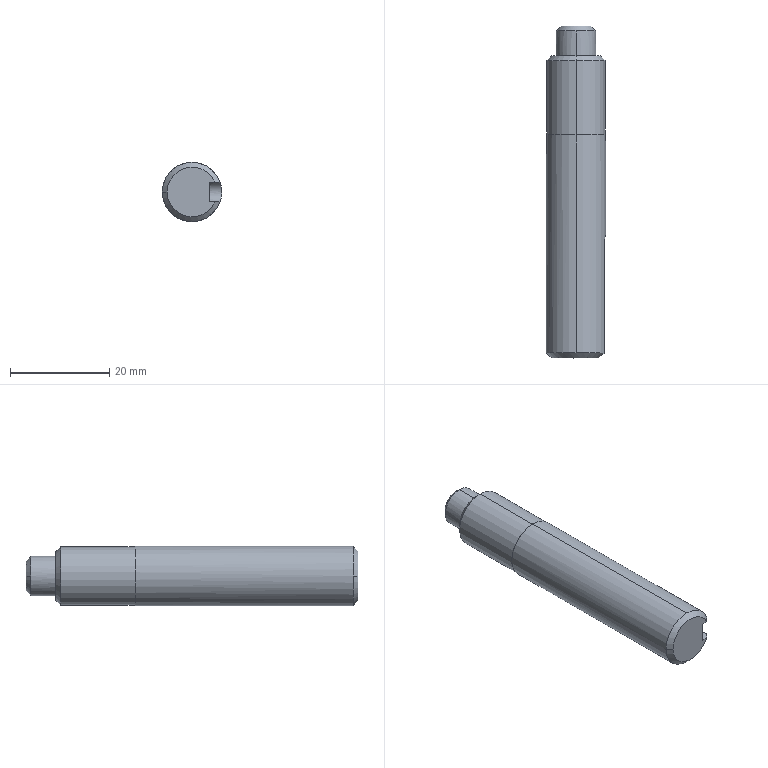Part | STEP file | 1 solid | 20 faces | box 12 x 67 x 12 mm | volume 6861 mm3 | cylinder 7 | plane 7 | cone 6 | commonest cylinder face diameters 8 x2 11.8 x2 12 x2 4 x1